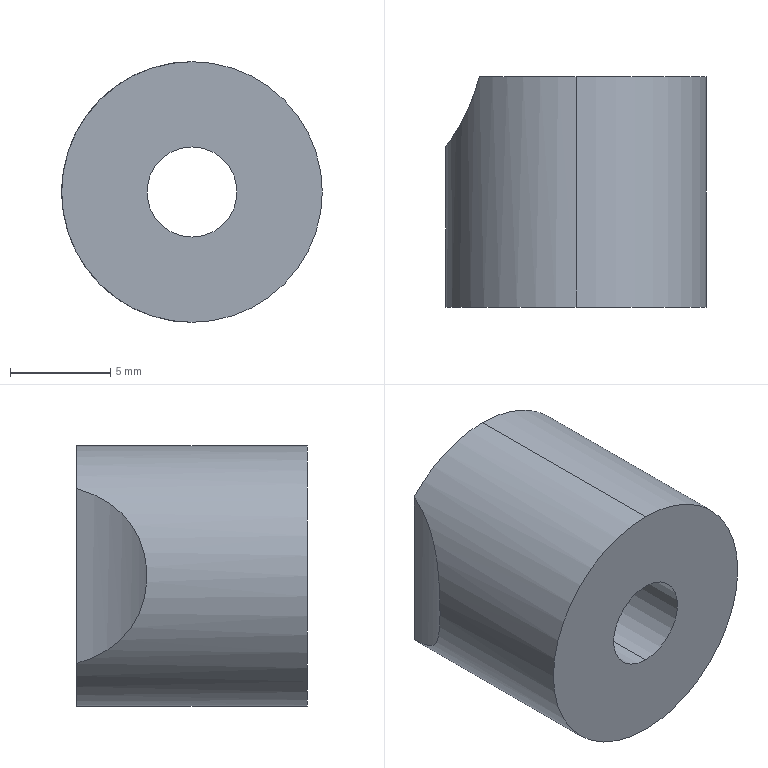Part | STEP file | BU-A15c | 1 solid | 7 faces | box 13 x 11.5 x 13 mm | volume 1326 mm3 | cylinder 5 | plane 2 | commonest cylinder face diameters 4.5 x2 13 x2 20 x1
STEP:
#1=CARTESIAN_POINT('',(0.,0.,0.));
#2=DIRECTION('',(0.,0.,1.));
#3=DIRECTION('',(1.,0.,0.));
#4=AXIS2_PLACEMENT_3D('',#1,#2,#3);
#5=CARTESIAN_POINT('',(0.,11.5,-2.25));
#6=VERTEX_POINT('',#5);
#7=CARTESIAN_POINT('',(0.,0.,-2.25));
#8=VERTEX_POINT('',#7);
#9=CARTESIAN_POINT('',(0.,0.,-2.25));
#10=DIRECTION('',(0.,-1.,0.));
#11=VECTOR('',#10,1.);
#12=LINE('',#9,#11);
#13=CARTESIAN_POINT('',(0.,0.,0.));
#14=DIRECTION('',(0.,-1.,0.));
#15=DIRECTION('',(0.,0.,-1.));
#16=AXIS2_PLACEMENT_3D('',#13,#14,#15);
#17=CYLINDRICAL_SURFACE('',#16,2.25);
#18=CARTESIAN_POINT('',(6.283,0.));
#19=DIRECTION('',(0.,1.));
#20=VECTOR('',#19,1.);
#21=LINE('',#18,#20);
#22=(GEOMETRIC_REPRESENTATION_CONTEXT(2)PARAMETRIC_REPRESENTATION_CONTEXT()REPRESENTATION_CONTEXT('',''));
#23=DEFINITIONAL_REPRESENTATION('',(#21),#22);
#24=PCURVE('',#17,#23);
#25=CARTESIAN_POINT('',(0.,0.,0.));
#26=DIRECTION('',(0.,-1.,0.));
#27=DIRECTION('',(0.,0.,-1.));
#28=AXIS2_PLACEMENT_3D('',#25,#26,#27);
#29=CYLINDRICAL_SURFACE('',#28,2.25);
#30=CARTESIAN_POINT('',(0.,0.));
#31=DIRECTION('',(0.,1.));
#32=VECTOR('',#31,1.);
#33=LINE('',#30,#32);
#34=(GEOMETRIC_REPRESENTATION_CONTEXT(2)PARAMETRIC_REPRESENTATION_CONTEXT()REPRESENTATION_CONTEXT('',''));
#35=DEFINITIONAL_REPRESENTATION('',(#33),#34);
#36=PCURVE('',#29,#35);
#37=SURFACE_CURVE('',#12,(#24,#36),.PCURVE_S1.);
#38=EDGE_CURVE('',#6,#8,#37,.T.);
#39=ORIENTED_EDGE('',*,*,#38,.T.);
#40=CARTESIAN_POINT('',(0.,0.,2.25));
#41=VERTEX_POINT('',#40);
#42=CARTESIAN_POINT('',(0.,0.,0.));
#43=DIRECTION('',(0.,-1.,0.));
#44=DIRECTION('',(0.,0.,-1.));
#45=AXIS2_PLACEMENT_3D('',#42,#43,#44);
#46=CIRCLE('',#45,2.25);
#47=CARTESIAN_POINT('',(0.,0.));
#48=DIRECTION('',(1.,0.));
#49=VECTOR('',#48,1.);
#50=LINE('',#47,#49);
#51=(GEOMETRIC_REPRESENTATION_CONTEXT(2)PARAMETRIC_REPRESENTATION_CONTEXT()REPRESENTATION_CONTEXT('',''));
#52=DEFINITIONAL_REPRESENTATION('',(#50),#51);
#53=PCURVE('',#17,#52);
#54=CARTESIAN_POINT('',(0.,0.,0.));
#55=DIRECTION('',(0.,1.,0.));
#56=DIRECTION('',(0.,0.,1.));
#57=AXIS2_PLACEMENT_3D('',#54,#55,#56);
#58=PLANE('',#57);
#59=CARTESIAN_POINT('',(-2.25,0.));
#60=CARTESIAN_POINT('',(-2.25,3.897));
#61=CARTESIAN_POINT('',(1.125,1.949));
#62=CARTESIAN_POINT('',(4.5,0.));
#63=CARTESIAN_POINT('',(1.125,-1.949));
#64=CARTESIAN_POINT('',(-2.25,-3.897));
#65=CARTESIAN_POINT('',(-2.25,0.));
#66=(BOUNDED_CURVE()B_SPLINE_CURVE(2,(#59,#60,#61,#62,#63,#64,#65),.UNSPECIFIED.,.T.,.F.)B_SPLINE_CURVE_WITH_KNOTS((1,2,2,2,2,1),(-2.094,0.,2.094,4.189,6.283,8.378),.UNSPECIFIED.)CURVE()GEOMETRIC_REPRESENTATION_ITEM()RATIONAL_B_SPLINE_CURVE((1.,0.5,1.,0.5,1.,0.5,1.))REPRESENTATION_ITEM(''));
#67=(GEOMETRIC_REPRESENTATION_CONTEXT(2)PARAMETRIC_REPRESENTATION_CONTEXT()REPRESENTATION_CONTEXT('',''));
#68=DEFINITIONAL_REPRESENTATION('',(#66),#67);
#69=PCURVE('',#58,#68);
#70=SURFACE_CURVE('',#46,(#53,#69),.PCURVE_S1.);
#71=EDGE_CURVE('',#41,#8,#70,.T.);
#72=ORIENTED_EDGE('',*,*,#71,.F.);
#73=CARTESIAN_POINT('',(0.,11.5,2.25));
#74=VERTEX_POINT('',#73);
#75=CARTESIAN_POINT('',(0.,0.,2.25));
#76=DIRECTION('',(0.,-1.,0.));
#77=VECTOR('',#76,1.);
#78=LINE('',#75,#77);
#79=CARTESIAN_POINT('',(3.142,0.));
#80=DIRECTION('',(0.,1.));
#81=VECTOR('',#80,1.);
#82=LINE('',#79,#81);
#83=(GEOMETRIC_REPRESENTATION_CONTEXT(2)PARAMETRIC_REPRESENTATION_CONTEXT()REPRESENTATION_CONTEXT('',''));
#84=DEFINITIONAL_REPRESENTATION('',(#82),#83);
#85=PCURVE('',#17,#84);
#86=CARTESIAN_POINT('',(3.142,0.));
#87=DIRECTION('',(0.,1.));
#88=VECTOR('',#87,1.);
#89=LINE('',#86,#88);
#90=(GEOMETRIC_REPRESENTATION_CONTEXT(2)PARAMETRIC_REPRESENTATION_CONTEXT()REPRESENTATION_CONTEXT('',''));
#91=DEFINITIONAL_REPRESENTATION('',(#89),#90);
#92=PCURVE('',#29,#91);
#93=SURFACE_CURVE('',#78,(#85,#92),.PCURVE_S1.);
#94=EDGE_CURVE('',#74,#41,#93,.T.);
#95=ORIENTED_EDGE('',*,*,#94,.F.);
#96=CARTESIAN_POINT('',(0.,11.5,0.));
#97=DIRECTION('',(0.,-1.,0.));
#98=DIRECTION('',(0.,0.,-1.));
#99=AXIS2_PLACEMENT_3D('',#96,#97,#98);
#100=CIRCLE('',#99,2.25);
#101=CARTESIAN_POINT('',(0.,-11.5));
#102=DIRECTION('',(1.,0.));
#103=VECTOR('',#102,1.);
#104=LINE('',#101,#103);
#105=(GEOMETRIC_REPRESENTATION_CONTEXT(2)PARAMETRIC_REPRESENTATION_CONTEXT()REPRESENTATION_CONTEXT('',''));
#106=DEFINITIONAL_REPRESENTATION('',(#104),#105);
#107=PCURVE('',#17,#106);
#108=CARTESIAN_POINT('',(0.,11.5,0.));
#109=DIRECTION('',(0.,-1.,0.));
#110=DIRECTION('',(0.,0.,-1.));
#111=AXIS2_PLACEMENT_3D('',#108,#109,#110);
#112=PLANE('',#111);
#113=CARTESIAN_POINT('',(0.,0.));
#114=DIRECTION('',(1.,0.));
#115=AXIS2_PLACEMENT_2D('',#113,#114);
#116=CIRCLE('',#115,2.25);
#117=(GEOMETRIC_REPRESENTATION_CONTEXT(2)PARAMETRIC_REPRESENTATION_CONTEXT()REPRESENTATION_CONTEXT('',''));
#118=DEFINITIONAL_REPRESENTATION('',(#116),#117);
#119=PCURVE('',#112,#118);
#120=SURFACE_CURVE('',#100,(#107,#119),.PCURVE_S1.);
#121=EDGE_CURVE('',#74,#6,#120,.T.);
#122=ORIENTED_EDGE('',*,*,#121,.T.);
#123=EDGE_LOOP('',(#39,#72,#95,#122));
#124=FACE_BOUND('',#123,.F.);
#125=ADVANCED_FACE('',(#124),#17,.F.);
#126=CARTESIAN_POINT('',(0.,0.,6.5));
#127=VERTEX_POINT('',#126);
#128=CARTESIAN_POINT('',(0.,0.,-6.5));
#129=VERTEX_POINT('',#128);
#130=CARTESIAN_POINT('',(0.,0.,0.));
#131=DIRECTION('',(0.,1.,0.));
#132=DIRECTION('',(0.,0.,1.));
#133=AXIS2_PLACEMENT_3D('',#130,#131,#132);
#134=CIRCLE('',#133,6.5);
#135=CARTESIAN_POINT('',(0.,0.,0.));
#136=DIRECTION('',(0.,1.,0.));
#137=DIRECTION('',(0.,0.,1.));
#138=AXIS2_PLACEMENT_3D('',#135,#136,#137);
#139=CYLINDRICAL_SURFACE('',#138,6.5);
#140=CARTESIAN_POINT('',(0.,0.));
#141=DIRECTION('',(1.,0.));
#142=VECTOR('',#141,1.);
#143=LINE('',#140,#142);
#144=(GEOMETRIC_REPRESENTATION_CONTEXT(2)PARAMETRIC_REPRESENTATION_CONTEXT()REPRESENTATION_CONTEXT('',''));
#145=DEFINITIONAL_REPRESENTATION('',(#143),#144);
#146=PCURVE('',#139,#145);
#147=CARTESIAN_POINT('',(0.,0.));
#148=DIRECTION('',(1.,0.));
#149=AXIS2_PLACEMENT_2D('',#147,#148);
#150=CIRCLE('',#149,6.5);
#151=(GEOMETRIC_REPRESENTATION_CONTEXT(2)PARAMETRIC_REPRESENTATION_CONTEXT()REPRESENTATION_CONTEXT('',''));
#152=DEFINITIONAL_REPRESENTATION('',(#150),#151);
#153=PCURVE('',#58,#152);
#154=SURFACE_CURVE('',#134,(#146,#153),.PCURVE_S1.);
#155=EDGE_CURVE('',#127,#129,#154,.T.);
#156=ORIENTED_EDGE('',*,*,#155,.T.);
#157=CARTESIAN_POINT('',(0.,11.5,-6.5));
#158=VERTEX_POINT('',#157);
#159=CARTESIAN_POINT('',(0.,0.,-6.5));
#160=DIRECTION('',(0.,1.,0.));
#161=VECTOR('',#160,1.);
#162=LINE('',#159,#161);
#163=CARTESIAN_POINT('',(3.142,0.));
#164=DIRECTION('',(0.,1.));
#165=VECTOR('',#164,1.);
#166=LINE('',#163,#165);
#167=(GEOMETRIC_REPRESENTATION_CONTEXT(2)PARAMETRIC_REPRESENTATION_CONTEXT()REPRESENTATION_CONTEXT('',''));
#168=DEFINITIONAL_REPRESENTATION('',(#166),#167);
#169=PCURVE('',#139,#168);
#170=CARTESIAN_POINT('',(0.,0.,0.));
#171=DIRECTION('',(0.,1.,0.));
#172=DIRECTION('',(0.,0.,1.));
#173=AXIS2_PLACEMENT_3D('',#170,#171,#172);
#174=CYLINDRICAL_SURFACE('',#173,6.5);
#175=CARTESIAN_POINT('',(3.142,0.));
#176=DIRECTION('',(0.,1.));
#177=VECTOR('',#176,1.);
#178=LINE('',#175,#177);
#179=(GEOMETRIC_REPRESENTATION_CONTEXT(2)PARAMETRIC_REPRESENTATION_CONTEXT()REPRESENTATION_CONTEXT('',''));
#180=DEFINITIONAL_REPRESENTATION('',(#178),#179);
#181=PCURVE('',#174,#180);
#182=SURFACE_CURVE('',#162,(#169,#181),.PCURVE_S1.);
#183=EDGE_CURVE('',#129,#158,#182,.T.);
#184=ORIENTED_EDGE('',*,*,#183,.T.);
#185=CARTESIAN_POINT('',(0.,11.5,6.5));
#186=VERTEX_POINT('',#185);
#187=CARTESIAN_POINT('',(0.,11.5,0.));
#188=DIRECTION('',(0.,1.,0.));
#189=DIRECTION('',(0.,0.,1.));
#190=AXIS2_PLACEMENT_3D('',#187,#188,#189);
#191=CIRCLE('',#190,6.5);
#192=CARTESIAN_POINT('',(0.,11.5));
#193=DIRECTION('',(1.,0.));
#194=VECTOR('',#193,1.);
#195=LINE('',#192,#194);
#196=(GEOMETRIC_REPRESENTATION_CONTEXT(2)PARAMETRIC_REPRESENTATION_CONTEXT()REPRESENTATION_CONTEXT('',''));
#197=DEFINITIONAL_REPRESENTATION('',(#195),#196);
#198=PCURVE('',#139,#197);
#199=CARTESIAN_POINT('',(-6.5,0.));
#200=CARTESIAN_POINT('',(-6.5,11.258));
#201=CARTESIAN_POINT('',(3.25,5.629));
#202=CARTESIAN_POINT('',(13.,0.));
#203=CARTESIAN_POINT('',(3.25,-5.629));
#204=CARTESIAN_POINT('',(-6.5,-11.258));
#205=CARTESIAN_POINT('',(-6.5,0.));
#206=(BOUNDED_CURVE()B_SPLINE_CURVE(2,(#199,#200,#201,#202,#203,#204,#205),.UNSPECIFIED.,.T.,.F.)B_SPLINE_CURVE_WITH_KNOTS((1,2,2,2,2,1),(-2.094,0.,2.094,4.189,6.283,8.378),.UNSPECIFIED.)CURVE()GEOMETRIC_REPRESENTATION_ITEM()RATIONAL_B_SPLINE_CURVE((1.,0.5,1.,0.5,1.,0.5,1.))REPRESENTATION_ITEM(''));
#207=(GEOMETRIC_REPRESENTATION_CONTEXT(2)PARAMETRIC_REPRESENTATION_CONTEXT()REPRESENTATION_CONTEXT('',''));
#208=DEFINITIONAL_REPRESENTATION('',(#206),#207);
#209=PCURVE('',#112,#208);
#210=SURFACE_CURVE('',#191,(#198,#209),.PCURVE_S1.);
#211=EDGE_CURVE('',#186,#158,#210,.T.);
#212=ORIENTED_EDGE('',*,*,#211,.F.);
#213=CARTESIAN_POINT('',(0.,0.,6.5));
#214=DIRECTION('',(0.,1.,0.));
#215=VECTOR('',#214,1.);
#216=LINE('',#213,#215);
#217=CARTESIAN_POINT('',(0.,0.));
#218=DIRECTION('',(0.,1.));
#219=VECTOR('',#218,1.);
#220=LINE('',#217,#219);
#221=(GEOMETRIC_REPRESENTATION_CONTEXT(2)PARAMETRIC_REPRESENTATION_CONTEXT()REPRESENTATION_CONTEXT('',''));
#222=DEFINITIONAL_REPRESENTATION('',(#220),#221);
#223=PCURVE('',#139,#222);
#224=CARTESIAN_POINT('',(6.283,0.));
#225=DIRECTION('',(0.,1.));
#226=VECTOR('',#225,1.);
#227=LINE('',#224,#226);
#228=(GEOMETRIC_REPRESENTATION_CONTEXT(2)PARAMETRIC_REPRESENTATION_CONTEXT()REPRESENTATION_CONTEXT('',''));
#229=DEFINITIONAL_REPRESENTATION('',(#227),#228);
#230=PCURVE('',#174,#229);
#231=SURFACE_CURVE('',#216,(#223,#230),.PCURVE_S1.);
#232=EDGE_CURVE('',#127,#186,#231,.T.);
#233=ORIENTED_EDGE('',*,*,#232,.F.);
#234=EDGE_LOOP('',(#156,#184,#212,#233));
#235=FACE_BOUND('',#234,.T.);
#236=ADVANCED_FACE('',(#235),#139,.T.);
#237=CARTESIAN_POINT('',(0.,11.5,0.));
#238=DIRECTION('',(0.,-1.,0.));
#239=DIRECTION('',(0.,0.,-1.));
#240=AXIS2_PLACEMENT_3D('',#237,#238,#239);
#241=CIRCLE('',#240,2.25);
#242=CARTESIAN_POINT('',(0.,0.));
#243=DIRECTION('',(1.,0.));
#244=AXIS2_PLACEMENT_2D('',#242,#243);
#245=CIRCLE('',#244,2.25);
#246=(GEOMETRIC_REPRESENTATION_CONTEXT(2)PARAMETRIC_REPRESENTATION_CONTEXT()REPRESENTATION_CONTEXT('',''));
#247=DEFINITIONAL_REPRESENTATION('',(#245),#246);
#248=PCURVE('',#112,#247);
#249=CARTESIAN_POINT('',(0.,-11.5));
#250=DIRECTION('',(1.,0.));
#251=VECTOR('',#250,1.);
#252=LINE('',#249,#251);
#253=(GEOMETRIC_REPRESENTATION_CONTEXT(2)PARAMETRIC_REPRESENTATION_CONTEXT()REPRESENTATION_CONTEXT('',''));
#254=DEFINITIONAL_REPRESENTATION('',(#252),#253);
#255=PCURVE('',#29,#254);
#256=SURFACE_CURVE('',#241,(#248,#255),.PCURVE_S1.);
#257=EDGE_CURVE('',#6,#74,#256,.T.);
#258=ORIENTED_EDGE('',*,*,#257,.T.);
#259=ORIENTED_EDGE('',*,*,#121,.T.);
#260=EDGE_LOOP('',(#258,#259));
#261=FACE_BOUND('',#260,.T.);
#262=CARTESIAN_POINT('',(-4.818,11.5,4.364));
#263=VERTEX_POINT('',#262);
#264=CARTESIAN_POINT('',(0.,11.5,0.));
#265=DIRECTION('',(0.,1.,0.));
#266=DIRECTION('',(0.,0.,1.));
#267=AXIS2_PLACEMENT_3D('',#264,#265,#266);
#268=CIRCLE('',#267,6.5);
#269=CARTESIAN_POINT('',(-6.5,0.));
#270=CARTESIAN_POINT('',(-6.5,11.258));
#271=CARTESIAN_POINT('',(3.25,5.629));
#272=CARTESIAN_POINT('',(13.,0.));
#273=CARTESIAN_POINT('',(3.25,-5.629));
#274=CARTESIAN_POINT('',(-6.5,-11.258));
#275=CARTESIAN_POINT('',(-6.5,0.));
#276=(BOUNDED_CURVE()B_SPLINE_CURVE(2,(#269,#270,#271,#272,#273,#274,#275),.UNSPECIFIED.,.T.,.F.)B_SPLINE_CURVE_WITH_KNOTS((1,2,2,2,2,1),(-2.094,0.,2.094,4.189,6.283,8.378),.UNSPECIFIED.)CURVE()GEOMETRIC_REPRESENTATION_ITEM()RATIONAL_B_SPLINE_CURVE((1.,0.5,1.,0.5,1.,0.5,1.))REPRESENTATION_ITEM(''));
#277=(GEOMETRIC_REPRESENTATION_CONTEXT(2)PARAMETRIC_REPRESENTATION_CONTEXT()REPRESENTATION_CONTEXT('',''));
#278=DEFINITIONAL_REPRESENTATION('',(#276),#277);
#279=PCURVE('',#112,#278);
#280=CARTESIAN_POINT('',(0.,11.5));
#281=DIRECTION('',(1.,0.));
#282=VECTOR('',#281,1.);
#283=LINE('',#280,#282);
#284=(GEOMETRIC_REPRESENTATION_CONTEXT(2)PARAMETRIC_REPRESENTATION_CONTEXT()REPRESENTATION_CONTEXT('',''));
#285=DEFINITIONAL_REPRESENTATION('',(#283),#284);
#286=PCURVE('',#174,#285);
#287=SURFACE_CURVE('',#268,(#279,#286),.PCURVE_S1.);
#288=EDGE_CURVE('',#263,#186,#287,.T.);
#289=ORIENTED_EDGE('',*,*,#288,.T.);
#290=ORIENTED_EDGE('',*,*,#211,.T.);
#291=CARTESIAN_POINT('',(-4.818,11.5,-4.364));
#292=VERTEX_POINT('',#291);
#293=CARTESIAN_POINT('',(0.,11.5,0.));
#294=DIRECTION('',(0.,1.,0.));
#295=DIRECTION('',(0.,0.,1.));
#296=AXIS2_PLACEMENT_3D('',#293,#294,#295);
#297=CIRCLE('',#296,6.5);
#298=CARTESIAN_POINT('',(-6.5,0.));
#299=CARTESIAN_POINT('',(-6.5,11.258));
#300=CARTESIAN_POINT('',(3.25,5.629));
#301=CARTESIAN_POINT('',(13.,0.));
#302=CARTESIAN_POINT('',(3.25,-5.629));
#303=CARTESIAN_POINT('',(-6.5,-11.258));
#304=CARTESIAN_POINT('',(-6.5,0.));
#305=(BOUNDED_CURVE()B_SPLINE_CURVE(2,(#298,#299,#300,#301,#302,#303,#304),.UNSPECIFIED.,.T.,.F.)B_SPLINE_CURVE_WITH_KNOTS((1,2,2,2,2,1),(-2.094,0.,2.094,4.189,6.283,8.378),.UNSPECIFIED.)CURVE()GEOMETRIC_REPRESENTATION_ITEM()RATIONAL_B_SPLINE_CURVE((1.,0.5,1.,0.5,1.,0.5,1.))REPRESENTATION_ITEM(''));
#306=(GEOMETRIC_REPRESENTATION_CONTEXT(2)PARAMETRIC_REPRESENTATION_CONTEXT()REPRESENTATION_CONTEXT('',''));
#307=DEFINITIONAL_REPRESENTATION('',(#305),#306);
#308=PCURVE('',#112,#307);
#309=CARTESIAN_POINT('',(0.,11.5));
#310=DIRECTION('',(1.,0.));
#311=VECTOR('',#310,1.);
#312=LINE('',#309,#311);
#313=(GEOMETRIC_REPRESENTATION_CONTEXT(2)PARAMETRIC_REPRESENTATION_CONTEXT()REPRESENTATION_CONTEXT('',''));
#314=DEFINITIONAL_REPRESENTATION('',(#312),#313);
#315=PCURVE('',#174,#314);
#316=SURFACE_CURVE('',#297,(#308,#315),.PCURVE_S1.);
#317=EDGE_CURVE('',#158,#292,#316,.T.);
#318=ORIENTED_EDGE('',*,*,#317,.T.);
#319=CARTESIAN_POINT('',(-4.818,11.5,-6.5));
#320=DIRECTION('',(0.,0.,1.));
#321=VECTOR('',#320,1.);
#322=LINE('',#319,#321);
#323=CARTESIAN_POINT('',(6.5,-4.818));
#324=DIRECTION('',(-1.,0.));
#325=VECTOR('',#324,1.);
#326=LINE('',#323,#325);
#327=(GEOMETRIC_REPRESENTATION_CONTEXT(2)PARAMETRIC_REPRESENTATION_CONTEXT()REPRESENTATION_CONTEXT('',''));
#328=DEFINITIONAL_REPRESENTATION('',(#326),#327);
#329=PCURVE('',#112,#328);
#330=CARTESIAN_POINT('',(-14.5,14.,-6.5));
#331=DIRECTION('',(0.,0.,1.));
#332=DIRECTION('',(1.,0.,0.));
#333=AXIS2_PLACEMENT_3D('',#330,#331,#332);
#334=CYLINDRICAL_SURFACE('',#333,10.);
#335=CARTESIAN_POINT('',(6.031,0.));
#336=DIRECTION('',(0.,1.));
#337=VECTOR('',#336,1.);
#338=LINE('',#335,#337);
#339=(GEOMETRIC_REPRESENTATION_CONTEXT(2)PARAMETRIC_REPRESENTATION_CONTEXT()REPRESENTATION_CONTEXT('',''));
#340=DEFINITIONAL_REPRESENTATION('',(#338),#339);
#341=PCURVE('',#334,#340);
#342=SURFACE_CURVE('',#322,(#329,#341),.PCURVE_S1.);
#343=EDGE_CURVE('',#292,#263,#342,.T.);
#344=ORIENTED_EDGE('',*,*,#343,.T.);
#345=EDGE_LOOP('',(#289,#290,#318,#344));
#346=FACE_BOUND('',#345,.T.);
#347=ADVANCED_FACE('',(#261,#346),#112,.F.);
#348=ORIENTED_EDGE('',*,*,#183,.F.);
#349=CARTESIAN_POINT('',(0.,0.,0.));
#350=DIRECTION('',(0.,1.,0.));
#351=DIRECTION('',(0.,0.,1.));
#352=AXIS2_PLACEMENT_3D('',#349,#350,#351);
#353=CIRCLE('',#352,6.5);
#354=CARTESIAN_POINT('',(0.,0.));
#355=DIRECTION('',(1.,0.));
#356=VECTOR('',#355,1.);
#357=LINE('',#354,#356);
#358=(GEOMETRIC_REPRESENTATION_CONTEXT(2)PARAMETRIC_REPRESENTATION_CONTEXT()REPRESENTATION_CONTEXT('',''));
#359=DEFINITIONAL_REPRESENTATION('',(#357),#358);
#360=PCURVE('',#174,#359);
#361=CARTESIAN_POINT('',(0.,0.));
#362=DIRECTION('',(1.,0.));
#363=AXIS2_PLACEMENT_2D('',#361,#362);
#364=CIRCLE('',#363,6.5);
#365=(GEOMETRIC_REPRESENTATION_CONTEXT(2)PARAMETRIC_REPRESENTATION_CONTEXT()REPRESENTATION_CONTEXT('',''));
#366=DEFINITIONAL_REPRESENTATION('',(#364),#365);
#367=PCURVE('',#58,#366);
#368=SURFACE_CURVE('',#353,(#360,#367),.PCURVE_S1.);
#369=EDGE_CURVE('',#129,#127,#368,.T.);
#370=ORIENTED_EDGE('',*,*,#369,.T.);
#371=ORIENTED_EDGE('',*,*,#232,.T.);
#372=ORIENTED_EDGE('',*,*,#288,.F.);
#373=CARTESIAN_POINT('',(-4.818,11.5,4.364));
#374=CARTESIAN_POINT('',(-4.945,11.006,4.223));
#375=CARTESIAN_POINT('',(-5.105,10.544,4.036));
#376=CARTESIAN_POINT('',(-5.374,9.904,3.659));
#377=CARTESIAN_POINT('',(-5.469,9.7,3.517));
#378=CARTESIAN_POINT('',(-5.657,9.325,3.206));
#379=CARTESIAN_POINT('',(-5.752,9.152,3.035));
#380=CARTESIAN_POINT('',(-5.934,8.837,2.66));
#381=CARTESIAN_POINT('',(-6.024,8.692,2.454));
#382=CARTESIAN_POINT('',(-6.183,8.446,2.018));
#383=CARTESIAN_POINT('',(-6.254,8.342,1.789));
#384=CARTESIAN_POINT('',(-6.372,8.174,1.309));
#385=CARTESIAN_POINT('',(-6.419,8.109,1.054));
#386=CARTESIAN_POINT('',(-6.483,8.023,0.5378));
#387=CARTESIAN_POINT('',(-6.499,8.001,0.2774));
#388=CARTESIAN_POINT('',(-6.501,7.999,-0.2484));
#389=CARTESIAN_POINT('',(-6.485,8.02,-0.5153));
#390=CARTESIAN_POINT('',(-6.423,8.104,-1.03));
#391=CARTESIAN_POINT('',(-6.377,8.166,-1.281));
#392=CARTESIAN_POINT('',(-6.259,8.334,-1.77));
#393=CARTESIAN_POINT('',(-6.188,8.438,-2.003));
#394=CARTESIAN_POINT('',(-6.029,8.683,-2.439));
#395=CARTESIAN_POINT('',(-5.941,8.825,-2.646));
#396=CARTESIAN_POINT('',(-5.757,9.143,-3.026));
#397=CARTESIAN_POINT('',(-5.662,9.317,-3.198));
#398=CARTESIAN_POINT('',(-5.472,9.694,-3.513));
#399=CARTESIAN_POINT('',(-5.377,9.898,-3.655));
#400=CARTESIAN_POINT('',(-5.107,10.538,-4.033));
#401=CARTESIAN_POINT('',(-4.945,11.005,-4.223));
#402=CARTESIAN_POINT('',(-4.818,11.5,-4.364));
#403=B_SPLINE_CURVE_WITH_KNOTS('',3,(#373,#374,#375,#376,#377,#378,#379,#380,#381,#382,#383,#384,#385,#386,#387,#388,#389,#390,#391,#392,#393,#394,#395,#396,#397,#398,#399,#400,#401,#402),.UNSPECIFIED.,.F.,.F.,(4,2,2,2,2,2,2,2,2,2,2,2,2,2,4),(0.,0.00157,0.002355,0.00314,0.003925,0.004709,0.005494,0.006279,0.007064,0.007849,0.008634,0.009419,0.0102,0.01099,0.01256),.UNSPECIFIED.);
#404=CARTESIAN_POINT('',(5.448,11.5));
#405=CARTESIAN_POINT('',(5.445,11.44));
#406=CARTESIAN_POINT('',(5.438,11.321));
#407=CARTESIAN_POINT('',(5.426,11.146));
#408=CARTESIAN_POINT('',(5.413,10.974));
#409=CARTESIAN_POINT('',(5.4,10.804));
#410=CARTESIAN_POINT('',(5.386,10.637));
#411=CARTESIAN_POINT('',(5.371,10.474));
#412=CARTESIAN_POINT('',(5.355,10.313));
#413=CARTESIAN_POINT('',(5.338,10.156));
#414=CARTESIAN_POINT('',(5.321,10.001));
#415=CARTESIAN_POINT('',(5.302,9.851));
#416=CARTESIAN_POINT('',(5.283,9.704));
#417=CARTESIAN_POINT('',(5.264,9.563));
#418=CARTESIAN_POINT('',(5.243,9.428));
#419=CARTESIAN_POINT('',(5.222,9.297));
#420=CARTESIAN_POINT('',(5.2,9.172));
#421=CARTESIAN_POINT('',(5.178,9.052));
#422=CARTESIAN_POINT('',(5.154,8.937));
#423=CARTESIAN_POINT('',(5.13,8.827));
#424=CARTESIAN_POINT('',(5.105,8.723));
#425=CARTESIAN_POINT('',(5.08,8.625));
#426=CARTESIAN_POINT('',(5.054,8.535));
#427=CARTESIAN_POINT('',(5.028,8.451));
#428=CARTESIAN_POINT('',(5.001,8.374));
#429=CARTESIAN_POINT('',(4.974,8.305));
#430=CARTESIAN_POINT('',(4.946,8.242));
#431=CARTESIAN_POINT('',(4.918,8.186));
#432=CARTESIAN_POINT('',(4.889,8.137));
#433=CARTESIAN_POINT('',(4.861,8.095));
#434=CARTESIAN_POINT('',(4.831,8.061));
#435=CARTESIAN_POINT('',(4.802,8.034));
#436=CARTESIAN_POINT('',(4.773,8.015));
#437=CARTESIAN_POINT('',(4.744,8.003));
#438=CARTESIAN_POINT('',(4.715,7.999));
#439=CARTESIAN_POINT('',(4.685,8.002));
#440=CARTESIAN_POINT('',(4.656,8.013));
#441=CARTESIAN_POINT('',(4.626,8.031));
#442=CARTESIAN_POINT('',(4.597,8.057));
#443=CARTESIAN_POINT('',(4.568,8.09));
#444=CARTESIAN_POINT('',(4.539,8.131));
#445=CARTESIAN_POINT('',(4.511,8.178));
#446=CARTESIAN_POINT('',(4.482,8.234));
#447=CARTESIAN_POINT('',(4.454,8.297));
#448=CARTESIAN_POINT('',(4.427,8.367));
#449=CARTESIAN_POINT('',(4.4,8.443));
#450=CARTESIAN_POINT('',(4.373,8.527));
#451=CARTESIAN_POINT('',(4.347,8.616));
#452=CARTESIAN_POINT('',(4.322,8.713));
#453=CARTESIAN_POINT('',(4.297,8.817));
#454=CARTESIAN_POINT('',(4.273,8.926));
#455=CARTESIAN_POINT('',(4.249,9.042));
#456=CARTESIAN_POINT('',(4.226,9.163));
#457=CARTESIAN_POINT('',(4.204,9.289));
#458=CARTESIAN_POINT('',(4.183,9.42));
#459=CARTESIAN_POINT('',(4.162,9.557));
#460=CARTESIAN_POINT('',(4.142,9.698));
#461=CARTESIAN_POINT('',(4.123,9.845));
#462=CARTESIAN_POINT('',(4.105,9.996));
#463=CARTESIAN_POINT('',(4.087,10.15));
#464=CARTESIAN_POINT('',(4.07,10.308));
#465=CARTESIAN_POINT('',(4.055,10.469));
#466=CARTESIAN_POINT('',(4.039,10.633));
#467=CARTESIAN_POINT('',(4.025,10.801));
#468=CARTESIAN_POINT('',(4.012,10.971));
#469=CARTESIAN_POINT('',(3.999,11.145));
#470=CARTESIAN_POINT('',(3.987,11.321));
#471=CARTESIAN_POINT('',(3.98,11.44));
#472=CARTESIAN_POINT('',(3.976,11.5));
#473=B_SPLINE_CURVE_WITH_KNOTS('',3,(#404,#405,#406,#407,#408,#409,#410,#411,#412,#413,#414,#415,#416,#417,#418,#419,#420,#421,#422,#423,#424,#425,#426,#427,#428,#429,#430,#431,#432,#433,#434,#435,#436,#437,#438,#439,#440,#441,#442,#443,#444,#445,#446,#447,#448,#449,#450,#451,#452,#453,#454,#455,#456,#457,#458,#459,#460,#461,#462,#463,#464,#465,#466,#467,#468,#469,#470,#471,#472),.UNSPECIFIED.,.F.,.F.,(4,1,1,1,1,1,1,1,1,1,1,1,1,1,1,1,1,1,1,1,1,1,1,1,1,1,1,1,1,1,1,1,1,1,1,1,1,1,1,1,1,1,1,1,1,1,1,1,1,1,1,1,1,1,1,1,1,1,1,1,1,1,1,1,1,1,4),(0.,0.0001903,0.0003806,0.0005708,0.0007611,0.0009514,0.001142,0.001332,0.001522,0.001713,0.001903,0.002093,0.002283,0.002474,0.002664,0.002854,0.003044,0.003235,0.003425,0.003615,0.003806,0.003996,0.004186,0.004376,0.004567,0.004757,0.004947,0.005138,0.005328,0.005518,0.005708,0.005899,0.006089,0.006279,0.006469,0.00666,0.00685,0.00704,0.007231,0.007421,0.007611,0.007801,0.007992,0.008182,0.008372,0.008563,0.008753,0.008943,0.009133,0.009324,0.009514,0.009704,0.009895,0.01008,0.01028,0.01047,0.01066,0.01085,0.01104,0.01123,0.01142,0.01161,0.0118,0.01199,0.01218,0.01237,0.01256),.QUASI_UNIFORM_KNOTS.);
#474=(GEOMETRIC_REPRESENTATION_CONTEXT(2)PARAMETRIC_REPRESENTATION_CONTEXT()REPRESENTATION_CONTEXT('',''));
#475=DEFINITIONAL_REPRESENTATION('',(#473),#474);
#476=PCURVE('',#174,#475);
#477=CARTESIAN_POINT('',(6.031,10.864));
#478=CARTESIAN_POINT('',(6.024,10.847));
#479=CARTESIAN_POINT('',(6.012,10.811));
#480=CARTESIAN_POINT('',(5.994,10.754));
#481=CARTESIAN_POINT('',(5.976,10.692));
#482=CARTESIAN_POINT('',(5.958,10.625));
#483=CARTESIAN_POINT('',(5.94,10.554));
#484=CARTESIAN_POINT('',(5.923,10.477));
#485=CARTESIAN_POINT('',(5.906,10.395));
#486=CARTESIAN_POINT('',(5.889,10.308));
#487=CARTESIAN_POINT('',(5.872,10.215));
#488=CARTESIAN_POINT('',(5.855,10.117));
#489=CARTESIAN_POINT('',(5.839,10.013));
#490=CARTESIAN_POINT('',(5.824,9.904));
#491=CARTESIAN_POINT('',(5.808,9.79));
#492=CARTESIAN_POINT('',(5.794,9.671));
#493=CARTESIAN_POINT('',(5.779,9.547));
#494=CARTESIAN_POINT('',(5.766,9.416));
#495=CARTESIAN_POINT('',(5.752,9.28));
#496=CARTESIAN_POINT('',(5.74,9.137));
#497=CARTESIAN_POINT('',(5.727,8.988));
#498=CARTESIAN_POINT('',(5.716,8.835));
#499=CARTESIAN_POINT('',(5.705,8.677));
#500=CARTESIAN_POINT('',(5.695,8.515));
#501=CARTESIAN_POINT('',(5.686,8.349));
#502=CARTESIAN_POINT('',(5.677,8.18));
#503=CARTESIAN_POINT('',(5.67,8.006));
#504=CARTESIAN_POINT('',(5.663,7.827));
#505=CARTESIAN_POINT('',(5.657,7.645));
#506=CARTESIAN_POINT('',(5.651,7.46));
#507=CARTESIAN_POINT('',(5.647,7.272));
#508=CARTESIAN_POINT('',(5.644,7.084));
#509=CARTESIAN_POINT('',(5.642,6.895));
#510=CARTESIAN_POINT('',(5.64,6.705));
#511=CARTESIAN_POINT('',(5.64,6.515));
#512=CARTESIAN_POINT('',(5.64,6.323));
#513=CARTESIAN_POINT('',(5.641,6.131));
#514=CARTESIAN_POINT('',(5.644,5.939));
#515=CARTESIAN_POINT('',(5.647,5.75));
#516=CARTESIAN_POINT('',(5.651,5.564));
#517=CARTESIAN_POINT('',(5.656,5.38));
#518=CARTESIAN_POINT('',(5.662,5.198));
#519=CARTESIAN_POINT('',(5.669,5.019));
#520=CARTESIAN_POINT('',(5.676,4.842));
#521=CARTESIAN_POINT('',(5.685,4.669));
#522=CARTESIAN_POINT('',(5.694,4.501));
#523=CARTESIAN_POINT('',(5.704,4.338));
#524=CARTESIAN_POINT('',(5.715,4.18));
#525=CARTESIAN_POINT('',(5.726,4.026));
#526=CARTESIAN_POINT('',(5.738,3.877));
#527=CARTESIAN_POINT('',(5.751,3.733));
#528=CARTESIAN_POINT('',(5.764,3.595));
#529=CARTESIAN_POINT('',(5.778,3.463));
#530=CARTESIAN_POINT('',(5.793,3.337));
#531=CARTESIAN_POINT('',(5.807,3.216));
#532=CARTESIAN_POINT('',(5.823,3.101));
#533=CARTESIAN_POINT('',(5.839,2.991));
#534=CARTESIAN_POINT('',(5.855,2.887));
#535=CARTESIAN_POINT('',(5.871,2.788));
#536=CARTESIAN_POINT('',(5.888,2.695));
#537=CARTESIAN_POINT('',(5.905,2.608));
#538=CARTESIAN_POINT('',(5.922,2.525));
#539=CARTESIAN_POINT('',(5.94,2.448));
#540=CARTESIAN_POINT('',(5.958,2.376));
#541=CARTESIAN_POINT('',(5.976,2.309));
#542=CARTESIAN_POINT('',(5.994,2.247));
#543=CARTESIAN_POINT('',(6.012,2.189));
#544=CARTESIAN_POINT('',(6.024,2.153));
#545=CARTESIAN_POINT('',(6.031,2.136));
#546=B_SPLINE_CURVE_WITH_KNOTS('',3,(#477,#478,#479,#480,#481,#482,#483,#484,#485,#486,#487,#488,#489,#490,#491,#492,#493,#494,#495,#496,#497,#498,#499,#500,#501,#502,#503,#504,#505,#506,#507,#508,#509,#510,#511,#512,#513,#514,#515,#516,#517,#518,#519,#520,#521,#522,#523,#524,#525,#526,#527,#528,#529,#530,#531,#532,#533,#534,#535,#536,#537,#538,#539,#540,#541,#542,#543,#544,#545),.UNSPECIFIED.,.F.,.F.,(4,1,1,1,1,1,1,1,1,1,1,1,1,1,1,1,1,1,1,1,1,1,1,1,1,1,1,1,1,1,1,1,1,1,1,1,1,1,1,1,1,1,1,1,1,1,1,1,1,1,1,1,1,1,1,1,1,1,1,1,1,1,1,1,1,1,4),(0.,0.0001903,0.0003806,0.0005708,0.0007611,0.0009514,0.001142,0.001332,0.001522,0.001713,0.001903,0.002093,0.002283,0.002474,0.002664,0.002854,0.003044,0.003235,0.003425,0.003615,0.003806,0.003996,0.004186,0.004376,0.004567,0.004757,0.004947,0.005138,0.005328,0.005518,0.005708,0.005899,0.006089,0.006279,0.006469,0.00666,0.00685,0.00704,0.007231,0.007421,0.007611,0.007801,0.007992,0.008182,0.008372,0.008563,0.008753,0.008943,0.009133,0.009324,0.009514,0.009704,0.009895,0.01008,0.01028,0.01047,0.01066,0.01085,0.01104,0.01123,0.01142,0.01161,0.0118,0.01199,0.01218,0.01237,0.01256),.QUASI_UNIFORM_KNOTS.);
#547=(GEOMETRIC_REPRESENTATION_CONTEXT(2)PARAMETRIC_REPRESENTATION_CONTEXT()REPRESENTATION_CONTEXT('',''));
#548=DEFINITIONAL_REPRESENTATION('',(#546),#547);
#549=PCURVE('',#334,#548);
#550=SURFACE_CURVE('',#403,(#476,#549),.PCURVE_S1.);
#551=EDGE_CURVE('',#263,#292,#550,.T.);
#552=ORIENTED_EDGE('',*,*,#551,.T.);
#553=ORIENTED_EDGE('',*,*,#317,.F.);
#554=EDGE_LOOP('',(#348,#370,#371,#372,#552,#553));
#555=FACE_BOUND('',#554,.T.);
#556=ADVANCED_FACE('',(#555),#174,.T.);
#557=CARTESIAN_POINT('',(0.,0.,0.));
#558=DIRECTION('',(0.,-1.,0.));
#559=DIRECTION('',(0.,0.,-1.));
#560=AXIS2_PLACEMENT_3D('',#557,#558,#559);
#561=CIRCLE('',#560,2.25);
#562=CARTESIAN_POINT('',(-2.25,0.));
#563=CARTESIAN_POINT('',(-2.25,3.897));
#564=CARTESIAN_POINT('',(1.125,1.949));
#565=CARTESIAN_POINT('',(4.5,0.));
#566=CARTESIAN_POINT('',(1.125,-1.949));
#567=CARTESIAN_POINT('',(-2.25,-3.897));
#568=CARTESIAN_POINT('',(-2.25,0.));
#569=(BOUNDED_CURVE()B_SPLINE_CURVE(2,(#562,#563,#564,#565,#566,#567,#568),.UNSPECIFIED.,.T.,.F.)B_SPLINE_CURVE_WITH_KNOTS((1,2,2,2,2,1),(-2.094,0.,2.094,4.189,6.283,8.378),.UNSPECIFIED.)CURVE()GEOMETRIC_REPRESENTATION_ITEM()RATIONAL_B_SPLINE_CURVE((1.,0.5,1.,0.5,1.,0.5,1.))REPRESENTATION_ITEM(''));
#570=(GEOMETRIC_REPRESENTATION_CONTEXT(2)PARAMETRIC_REPRESENTATION_CONTEXT()REPRESENTATION_CONTEXT('',''));
#571=DEFINITIONAL_REPRESENTATION('',(#569),#570);
#572=PCURVE('',#58,#571);
#573=CARTESIAN_POINT('',(0.,0.));
#574=DIRECTION('',(1.,0.));
#575=VECTOR('',#574,1.);
#576=LINE('',#573,#575);
#577=(GEOMETRIC_REPRESENTATION_CONTEXT(2)PARAMETRIC_REPRESENTATION_CONTEXT()REPRESENTATION_CONTEXT('',''));
#578=DEFINITIONAL_REPRESENTATION('',(#576),#577);
#579=PCURVE('',#29,#578);
#580=SURFACE_CURVE('',#561,(#572,#579),.PCURVE_S1.);
#581=EDGE_CURVE('',#8,#41,#580,.T.);
#582=ORIENTED_EDGE('',*,*,#581,.F.);
#583=ORIENTED_EDGE('',*,*,#71,.F.);
#584=EDGE_LOOP('',(#582,#583));
#585=FACE_BOUND('',#584,.T.);
#586=ORIENTED_EDGE('',*,*,#155,.F.);
#587=ORIENTED_EDGE('',*,*,#369,.F.);
#588=EDGE_LOOP('',(#586,#587));
#589=FACE_BOUND('',#588,.T.);
#590=ADVANCED_FACE('',(#585,#589),#58,.F.);
#591=ORIENTED_EDGE('',*,*,#551,.T.);
#592=ORIENTED_EDGE('',*,*,#343,.T.);
#593=EDGE_LOOP('',(#591,#592));
#594=FACE_BOUND('',#593,.F.);
#595=ADVANCED_FACE('',(#594),#334,.F.);
#596=ORIENTED_EDGE('',*,*,#581,.F.);
#597=ORIENTED_EDGE('',*,*,#38,.F.);
#598=ORIENTED_EDGE('',*,*,#257,.T.);
#599=ORIENTED_EDGE('',*,*,#94,.T.);
#600=EDGE_LOOP('',(#596,#597,#598,#599));
#601=FACE_BOUND('',#600,.F.);
#602=ADVANCED_FACE('',(#601),#29,.F.);
#603=CLOSED_SHELL('',(#125,#236,#347,#556,#590,#595,#602));
#604=MANIFOLD_SOLID_BREP('',#603);
#605=(LENGTH_UNIT()NAMED_UNIT(*)SI_UNIT(.MILLI.,.METRE.));
#606=UNCERTAINTY_MEASURE_WITH_UNIT(LENGTH_MEASURE(0.00002),#605,'','');
#607=(NAMED_UNIT(*)PLANE_ANGLE_UNIT()SI_UNIT($,.RADIAN.));
#608=(NAMED_UNIT(*)SI_UNIT($,.STERADIAN.)SOLID_ANGLE_UNIT());
#609=(GEOMETRIC_REPRESENTATION_CONTEXT(3)GLOBAL_UNCERTAINTY_ASSIGNED_CONTEXT((#606))GLOBAL_UNIT_ASSIGNED_CONTEXT((#605,#607,#608))REPRESENTATION_CONTEXT('',''));
#610=ADVANCED_BREP_SHAPE_REPRESENTATION('',(#4,#604),#609);